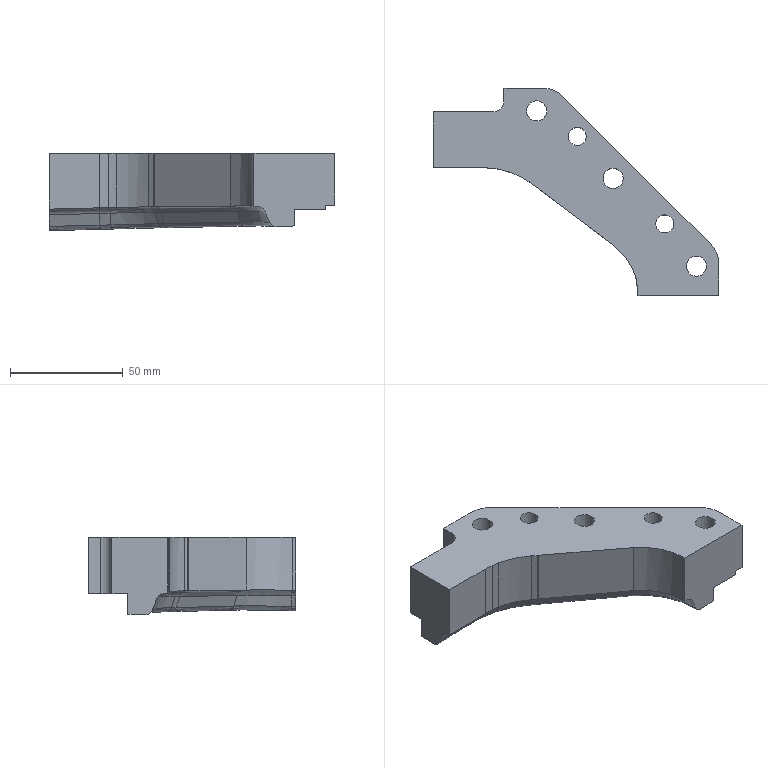Part | STEP file | 810_id1582_x_t | 1 solid | 70 faces | box 127 x 92 x 34.31 mm | volume 120451 mm3 | spline 34 | plane 21 | cylinder 14 | other 1 | commonest cylinder face diameters 9 x3 10 x3 14 x3 8 x2 24 x2 30 x1